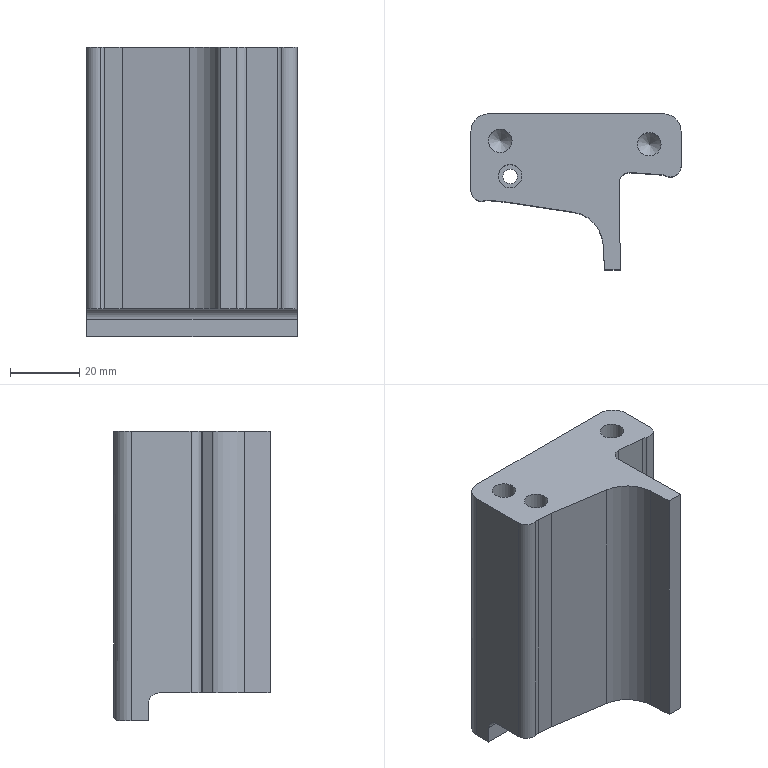Part | NX | features solid 2 | 1 solid | 32 faces | box 60.587 x 45.023 x 83.5 mm | volume 117737 mm3 | cylinder 15 | plane 14 | cone 3 | commonest cylinder face diameters 6 x6 6.8 x3 10 x2 2 x1 4.2 x1 5.2 x1
STEP:
#1=CARTESIAN_POINT('',(40.263,90.,-5.5));
#2=VERTEX_POINT('',#1);
#3=CARTESIAN_POINT('',(42.363,90.,-5.5));
#4=DIRECTION('',(0.,0.,-1.));
#5=DIRECTION('',(-1.,0.,0.));
#6=AXIS2_PLACEMENT_3D('',#3,#4,#5);
#7=CIRCLE('',#6,2.1);
#8=EDGE_CURVE('',#2,#2,#7,.T.);
#9=ORIENTED_EDGE('',*,*,#8,.F.);
#10=EDGE_LOOP('',(#9));
#11=FACE_BOUND('',#10,.T.);
#12=CARTESIAN_POINT('',(74.154,62.977,-5.5));
#13=VERTEX_POINT('',#12);
#14=CARTESIAN_POINT('',(69.599,62.977,-5.5));
#15=VERTEX_POINT('',#14);
#16=CARTESIAN_POINT('',(34.069,62.977,-5.5));
#17=DIRECTION('',(1.,0.,0.));
#18=VECTOR('',#17,1000.);
#19=LINE('',#16,#18);
#20=EDGE_CURVE('',#13,#15,#19,.F.);
#21=ORIENTED_EDGE('',*,*,#20,.T.);
#22=CARTESIAN_POINT('',(69.171,70.288,-5.5));
#23=VERTEX_POINT('',#22);
#24=CARTESIAN_POINT('',(69.651,62.096,-5.5));
#25=DIRECTION('',(-0.05848,0.9983,0.));
#26=VECTOR('',#25,1000.);
#27=LINE('',#24,#26);
#28=EDGE_CURVE('',#15,#23,#27,.T.);
#29=ORIENTED_EDGE('',*,*,#28,.T.);
#30=CARTESIAN_POINT('',(60.68,79.591,-5.5));
#31=VERTEX_POINT('',#30);
#32=CARTESIAN_POINT('',(59.188,69.703,-5.5));
#33=DIRECTION('',(0.,0.,1.));
#34=DIRECTION('',(1.,0.,0.));
#35=AXIS2_PLACEMENT_3D('',#32,#33,#34);
#36=CIRCLE('',#35,10.);
#37=EDGE_CURVE('',#23,#31,#36,.T.);
#38=ORIENTED_EDGE('',*,*,#37,.T.);
#39=CARTESIAN_POINT('',(41.179,82.535,-5.5));
#40=VERTEX_POINT('',#39);
#41=CARTESIAN_POINT('',(60.68,79.591,-5.5));
#42=DIRECTION('',(-0.9888,0.1493,0.));
#43=VECTOR('',#42,1000.);
#44=LINE('',#41,#43);
#45=EDGE_CURVE('',#31,#40,#44,.T.);
#46=ORIENTED_EDGE('',*,*,#45,.T.);
#47=CARTESIAN_POINT('',(36.197,83.04,-5.5));
#48=VERTEX_POINT('',#47);
#49=CARTESIAN_POINT('',(41.179,82.535,-5.5));
#50=DIRECTION('',(-0.9949,0.1009,0.));
#51=VECTOR('',#50,1000.);
#52=LINE('',#49,#51);
#53=EDGE_CURVE('',#40,#48,#52,.T.);
#54=ORIENTED_EDGE('',*,*,#53,.T.);
#55=CARTESIAN_POINT('',(34.982,82.913,-5.5));
#56=VERTEX_POINT('',#55);
#57=CARTESIAN_POINT('',(35.894,80.055,-5.5));
#58=DIRECTION('',(0.,0.,1.));
#59=DIRECTION('',(1.,0.,0.));
#60=AXIS2_PLACEMENT_3D('',#57,#58,#59);
#61=CIRCLE('',#60,3.);
#62=EDGE_CURVE('',#48,#56,#61,.T.);
#63=ORIENTED_EDGE('',*,*,#62,.T.);
#64=CARTESIAN_POINT('',(31.069,85.771,-5.5));
#65=VERTEX_POINT('',#64);
#66=CARTESIAN_POINT('',(34.069,85.771,-5.5));
#67=DIRECTION('',(0.,0.,-1.));
#68=DIRECTION('',(1.,0.,0.));
#69=AXIS2_PLACEMENT_3D('',#66,#67,#68);
#70=CIRCLE('',#69,3.);
#71=EDGE_CURVE('',#56,#65,#70,.T.);
#72=ORIENTED_EDGE('',*,*,#71,.T.);
#73=CARTESIAN_POINT('',(31.069,95.,-5.5));
#74=VERTEX_POINT('',#73);
#75=CARTESIAN_POINT('',(31.069,85.771,-5.5));
#76=DIRECTION('',(0.,1.,0.));
#77=VECTOR('',#76,1000.);
#78=LINE('',#75,#77);
#79=EDGE_CURVE('',#65,#74,#78,.T.);
#80=ORIENTED_EDGE('',*,*,#79,.T.);
#81=CARTESIAN_POINT('',(91.657,95.,-5.5));
#82=VERTEX_POINT('',#81);
#83=CARTESIAN_POINT('',(34.069,95.,-5.5));
#84=DIRECTION('',(1.,0.,0.));
#85=VECTOR('',#84,1000.);
#86=LINE('',#83,#85);
#87=EDGE_CURVE('',#74,#82,#86,.T.);
#88=ORIENTED_EDGE('',*,*,#87,.T.);
#89=CARTESIAN_POINT('',(91.657,92.731,-5.5));
#90=VERTEX_POINT('',#89);
#91=CARTESIAN_POINT('',(91.657,109.703,-5.5));
#92=DIRECTION('',(0.,-1.,0.));
#93=VECTOR('',#92,1000.);
#94=LINE('',#91,#93);
#95=EDGE_CURVE('',#82,#90,#94,.T.);
#96=ORIENTED_EDGE('',*,*,#95,.T.);
#97=CARTESIAN_POINT('',(87.27,90.071,-5.5));
#98=VERTEX_POINT('',#97);
#99=CARTESIAN_POINT('',(88.657,92.731,-5.5));
#100=DIRECTION('',(0.,0.,-1.));
#101=DIRECTION('',(1.,0.,0.));
#102=AXIS2_PLACEMENT_3D('',#99,#100,#101);
#103=CIRCLE('',#102,3.);
#104=EDGE_CURVE('',#90,#98,#103,.T.);
#105=ORIENTED_EDGE('',*,*,#104,.T.);
#106=CARTESIAN_POINT('',(86.093,90.403,-5.5));
#107=VERTEX_POINT('',#106);
#108=CARTESIAN_POINT('',(85.883,87.411,-5.5));
#109=DIRECTION('',(0.,0.,1.));
#110=DIRECTION('',(1.,0.,0.));
#111=AXIS2_PLACEMENT_3D('',#108,#109,#110);
#112=CIRCLE('',#111,3.);
#113=EDGE_CURVE('',#98,#107,#112,.T.);
#114=ORIENTED_EDGE('',*,*,#113,.T.);
#115=CARTESIAN_POINT('',(77.047,91.037,-5.5));
#116=VERTEX_POINT('',#115);
#117=CARTESIAN_POINT('',(86.093,90.403,-5.5));
#118=DIRECTION('',(-0.9976,0.06991,0.));
#119=VECTOR('',#118,1000.);
#120=LINE('',#117,#119);
#121=EDGE_CURVE('',#107,#116,#120,.T.);
#122=ORIENTED_EDGE('',*,*,#121,.T.);
#123=CARTESIAN_POINT('',(73.838,88.007,-5.5));
#124=VERTEX_POINT('',#123);
#125=CARTESIAN_POINT('',(76.838,88.044,-5.5));
#126=DIRECTION('',(0.,0.,1.));
#127=DIRECTION('',(1.,0.,0.));
#128=AXIS2_PLACEMENT_3D('',#125,#126,#127);
#129=CIRCLE('',#128,3.);
#130=EDGE_CURVE('',#116,#124,#129,.T.);
#131=ORIENTED_EDGE('',*,*,#130,.T.);
#132=CARTESIAN_POINT('',(73.838,88.007,-5.5));
#133=DIRECTION('',(0.01263,-0.9999,0.));
#134=VECTOR('',#133,1000.);
#135=LINE('',#132,#134);
#136=EDGE_CURVE('',#124,#13,#135,.T.);
#137=ORIENTED_EDGE('',*,*,#136,.T.);
#138=EDGE_LOOP('',(#21,#29,#38,#46,#54,#63,#72,#80,#88,#96,#105,#114,#122,#131,#137));
#139=FACE_BOUND('',#138,.T.);
#140=CARTESIAN_POINT('',(58.763,91.,-5.5));
#141=VERTEX_POINT('',#140);
#142=CARTESIAN_POINT('',(61.363,91.,-5.5));
#143=DIRECTION('',(0.,0.,-1.));
#144=DIRECTION('',(-1.,0.,0.));
#145=AXIS2_PLACEMENT_3D('',#142,#143,#144);
#146=CIRCLE('',#145,2.6);
#147=EDGE_CURVE('',#141,#141,#146,.F.);
#148=ORIENTED_EDGE('',*,*,#147,.T.);
#149=EDGE_LOOP('',(#148));
#150=FACE_BOUND('',#149,.T.);
#151=CARTESIAN_POINT('',(34.069,110.84,-5.5));
#152=DIRECTION('',(0.,0.,-1.));
#153=DIRECTION('',(-1.,0.,0.));
#154=AXIS2_PLACEMENT_3D('',#151,#152,#153);
#155=PLANE('',#154);
#156=ADVANCED_FACE('',(#11,#139,#150),#155,.T.);
#157=CARTESIAN_POINT('',(91.657,98.,-13.5));
#158=VERTEX_POINT('',#157);
#159=CARTESIAN_POINT('',(91.657,103.,-13.5));
#160=VERTEX_POINT('',#159);
#161=CARTESIAN_POINT('',(91.657,98.,-13.5));
#162=DIRECTION('',(0.,1.,0.));
#163=VECTOR('',#162,1000.);
#164=LINE('',#161,#163);
#165=EDGE_CURVE('',#158,#160,#164,.T.);
#166=ORIENTED_EDGE('',*,*,#165,.F.);
#167=CARTESIAN_POINT('',(31.069,98.,-13.5));
#168=VERTEX_POINT('',#167);
#169=CARTESIAN_POINT('',(34.069,98.,-13.5));
#170=DIRECTION('',(1.,0.,0.));
#171=VECTOR('',#170,1000.);
#172=LINE('',#169,#171);
#173=EDGE_CURVE('',#168,#158,#172,.T.);
#174=ORIENTED_EDGE('',*,*,#173,.F.);
#175=CARTESIAN_POINT('',(31.069,103.,-13.5));
#176=VERTEX_POINT('',#175);
#177=CARTESIAN_POINT('',(31.069,98.,-13.5));
#178=DIRECTION('',(0.,1.,0.));
#179=VECTOR('',#178,1000.);
#180=LINE('',#177,#179);
#181=EDGE_CURVE('',#168,#176,#180,.T.);
#182=ORIENTED_EDGE('',*,*,#181,.T.);
#183=CARTESIAN_POINT('',(33.069,107.,-13.5));
#184=VERTEX_POINT('',#183);
#185=CARTESIAN_POINT('',(36.069,103.,-13.5));
#186=DIRECTION('',(0.,0.,1.));
#187=DIRECTION('',(1.,0.,0.));
#188=AXIS2_PLACEMENT_3D('',#185,#186,#187);
#189=CIRCLE('',#188,5.);
#190=EDGE_CURVE('',#176,#184,#189,.F.);
#191=ORIENTED_EDGE('',*,*,#190,.T.);
#192=CARTESIAN_POINT('',(89.657,107.,-13.5));
#193=VERTEX_POINT('',#192);
#194=CARTESIAN_POINT('',(86.657,107.,-13.5));
#195=DIRECTION('',(-1.,0.,0.));
#196=VECTOR('',#195,1000.);
#197=LINE('',#194,#196);
#198=EDGE_CURVE('',#184,#193,#197,.F.);
#199=ORIENTED_EDGE('',*,*,#198,.T.);
#200=CARTESIAN_POINT('',(86.657,103.,-13.5));
#201=DIRECTION('',(0.,0.,1.));
#202=DIRECTION('',(1.,0.,0.));
#203=AXIS2_PLACEMENT_3D('',#200,#201,#202);
#204=CIRCLE('',#203,5.);
#205=EDGE_CURVE('',#193,#160,#204,.F.);
#206=ORIENTED_EDGE('',*,*,#205,.T.);
#207=EDGE_LOOP('',(#166,#174,#182,#191,#199,#206));
#208=FACE_BOUND('',#207,.T.);
#209=CARTESIAN_POINT('',(34.069,98.,-13.5));
#210=DIRECTION('',(0.,0.,1.));
#211=DIRECTION('',(1.,0.,0.));
#212=AXIS2_PLACEMENT_3D('',#209,#210,#211);
#213=PLANE('',#212);
#214=ADVANCED_FACE('',(#208),#213,.F.);
#215=CARTESIAN_POINT('',(42.9,100.2,70.));
#216=VERTEX_POINT('',#215);
#217=CARTESIAN_POINT('',(39.5,100.2,70.));
#218=DIRECTION('',(0.,0.,-1.));
#219=DIRECTION('',(1.,0.,0.));
#220=AXIS2_PLACEMENT_3D('',#217,#218,#219);
#221=CIRCLE('',#220,3.4);
#222=EDGE_CURVE('',#216,#216,#221,.T.);
#223=ORIENTED_EDGE('',*,*,#222,.T.);
#224=EDGE_LOOP('',(#223));
#225=FACE_BOUND('',#224,.T.);
#226=CARTESIAN_POINT('',(74.154,62.977,70.));
#227=VERTEX_POINT('',#226);
#228=CARTESIAN_POINT('',(69.599,62.977,70.));
#229=VERTEX_POINT('',#228);
#230=CARTESIAN_POINT('',(-37.5,62.977,70.));
#231=DIRECTION('',(-1.,0.,0.));
#232=VECTOR('',#231,1000.);
#233=LINE('',#230,#232);
#234=EDGE_CURVE('',#227,#229,#233,.T.);
#235=ORIENTED_EDGE('',*,*,#234,.F.);
#236=CARTESIAN_POINT('',(73.838,88.007,70.));
#237=VERTEX_POINT('',#236);
#238=CARTESIAN_POINT('',(73.838,88.007,70.));
#239=DIRECTION('',(0.01263,-0.9999,0.));
#240=VECTOR('',#239,1000.);
#241=LINE('',#238,#240);
#242=EDGE_CURVE('',#237,#227,#241,.T.);
#243=ORIENTED_EDGE('',*,*,#242,.F.);
#244=CARTESIAN_POINT('',(77.047,91.037,70.));
#245=VERTEX_POINT('',#244);
#246=CARTESIAN_POINT('',(76.838,88.044,70.));
#247=DIRECTION('',(0.,0.,1.));
#248=DIRECTION('',(1.,0.,0.));
#249=AXIS2_PLACEMENT_3D('',#246,#247,#248);
#250=CIRCLE('',#249,3.);
#251=EDGE_CURVE('',#245,#237,#250,.T.);
#252=ORIENTED_EDGE('',*,*,#251,.F.);
#253=CARTESIAN_POINT('',(86.093,90.403,70.));
#254=VERTEX_POINT('',#253);
#255=CARTESIAN_POINT('',(86.093,90.403,70.));
#256=DIRECTION('',(-0.9976,0.06991,0.));
#257=VECTOR('',#256,1000.);
#258=LINE('',#255,#257);
#259=EDGE_CURVE('',#254,#245,#258,.T.);
#260=ORIENTED_EDGE('',*,*,#259,.F.);
#261=CARTESIAN_POINT('',(87.27,90.071,70.));
#262=VERTEX_POINT('',#261);
#263=CARTESIAN_POINT('',(85.883,87.411,70.));
#264=DIRECTION('',(0.,0.,1.));
#265=DIRECTION('',(1.,0.,0.));
#266=AXIS2_PLACEMENT_3D('',#263,#264,#265);
#267=CIRCLE('',#266,3.);
#268=EDGE_CURVE('',#262,#254,#267,.T.);
#269=ORIENTED_EDGE('',*,*,#268,.F.);
#270=CARTESIAN_POINT('',(91.657,92.731,70.));
#271=VERTEX_POINT('',#270);
#272=CARTESIAN_POINT('',(88.657,92.731,70.));
#273=DIRECTION('',(0.,0.,1.));
#274=DIRECTION('',(1.,0.,0.));
#275=AXIS2_PLACEMENT_3D('',#272,#273,#274);
#276=CIRCLE('',#275,3.);
#277=EDGE_CURVE('',#271,#262,#276,.F.);
#278=ORIENTED_EDGE('',*,*,#277,.F.);
#279=CARTESIAN_POINT('',(91.657,103.,70.));
#280=VERTEX_POINT('',#279);
#281=CARTESIAN_POINT('',(91.657,109.703,70.));
#282=DIRECTION('',(0.,-1.,0.));
#283=VECTOR('',#282,1000.);
#284=LINE('',#281,#283);
#285=EDGE_CURVE('',#280,#271,#284,.T.);
#286=ORIENTED_EDGE('',*,*,#285,.F.);
#287=CARTESIAN_POINT('',(86.657,108.,70.));
#288=VERTEX_POINT('',#287);
#289=CARTESIAN_POINT('',(86.657,103.,70.));
#290=DIRECTION('',(0.,0.,1.));
#291=DIRECTION('',(1.,0.,0.));
#292=AXIS2_PLACEMENT_3D('',#289,#290,#291);
#293=CIRCLE('',#292,5.);
#294=EDGE_CURVE('',#288,#280,#293,.F.);
#295=ORIENTED_EDGE('',*,*,#294,.F.);
#296=CARTESIAN_POINT('',(36.069,108.,70.));
#297=VERTEX_POINT('',#296);
#298=CARTESIAN_POINT('',(34.069,108.,70.));
#299=DIRECTION('',(1.,0.,0.));
#300=VECTOR('',#299,1000.);
#301=LINE('',#298,#300);
#302=EDGE_CURVE('',#297,#288,#301,.T.);
#303=ORIENTED_EDGE('',*,*,#302,.F.);
#304=CARTESIAN_POINT('',(31.069,103.,70.));
#305=VERTEX_POINT('',#304);
#306=CARTESIAN_POINT('',(36.069,103.,70.));
#307=DIRECTION('',(0.,0.,1.));
#308=DIRECTION('',(1.,0.,0.));
#309=AXIS2_PLACEMENT_3D('',#306,#307,#308);
#310=CIRCLE('',#309,5.);
#311=EDGE_CURVE('',#305,#297,#310,.F.);
#312=ORIENTED_EDGE('',*,*,#311,.F.);
#313=CARTESIAN_POINT('',(31.069,85.771,70.));
#314=VERTEX_POINT('',#313);
#315=CARTESIAN_POINT('',(31.069,85.771,70.));
#316=DIRECTION('',(0.,1.,0.));
#317=VECTOR('',#316,1000.);
#318=LINE('',#315,#317);
#319=EDGE_CURVE('',#314,#305,#318,.T.);
#320=ORIENTED_EDGE('',*,*,#319,.F.);
#321=CARTESIAN_POINT('',(34.982,82.913,70.));
#322=VERTEX_POINT('',#321);
#323=CARTESIAN_POINT('',(34.069,85.771,70.));
#324=DIRECTION('',(0.,0.,1.));
#325=DIRECTION('',(1.,0.,0.));
#326=AXIS2_PLACEMENT_3D('',#323,#324,#325);
#327=CIRCLE('',#326,3.);
#328=EDGE_CURVE('',#322,#314,#327,.F.);
#329=ORIENTED_EDGE('',*,*,#328,.F.);
#330=CARTESIAN_POINT('',(36.197,83.04,70.));
#331=VERTEX_POINT('',#330);
#332=CARTESIAN_POINT('',(35.894,80.055,70.));
#333=DIRECTION('',(0.,0.,1.));
#334=DIRECTION('',(1.,0.,0.));
#335=AXIS2_PLACEMENT_3D('',#332,#333,#334);
#336=CIRCLE('',#335,3.);
#337=EDGE_CURVE('',#331,#322,#336,.T.);
#338=ORIENTED_EDGE('',*,*,#337,.F.);
#339=CARTESIAN_POINT('',(41.179,82.535,70.));
#340=VERTEX_POINT('',#339);
#341=CARTESIAN_POINT('',(41.179,82.535,70.));
#342=DIRECTION('',(-0.9949,0.1009,0.));
#343=VECTOR('',#342,1000.);
#344=LINE('',#341,#343);
#345=EDGE_CURVE('',#340,#331,#344,.T.);
#346=ORIENTED_EDGE('',*,*,#345,.F.);
#347=CARTESIAN_POINT('',(60.68,79.591,70.));
#348=VERTEX_POINT('',#347);
#349=CARTESIAN_POINT('',(60.68,79.591,70.));
#350=DIRECTION('',(-0.9888,0.1493,0.));
#351=VECTOR('',#350,1000.);
#352=LINE('',#349,#351);
#353=EDGE_CURVE('',#348,#340,#352,.T.);
#354=ORIENTED_EDGE('',*,*,#353,.F.);
#355=CARTESIAN_POINT('',(69.171,70.288,70.));
#356=VERTEX_POINT('',#355);
#357=CARTESIAN_POINT('',(59.188,69.703,70.));
#358=DIRECTION('',(0.,0.,1.));
#359=DIRECTION('',(1.,0.,0.));
#360=AXIS2_PLACEMENT_3D('',#357,#358,#359);
#361=CIRCLE('',#360,10.);
#362=EDGE_CURVE('',#348,#356,#361,.F.);
#363=ORIENTED_EDGE('',*,*,#362,.T.);
#364=CARTESIAN_POINT('',(69.651,62.096,70.));
#365=DIRECTION('',(-0.05848,0.9983,0.));
#366=VECTOR('',#365,1000.);
#367=LINE('',#364,#366);
#368=EDGE_CURVE('',#356,#229,#367,.F.);
#369=ORIENTED_EDGE('',*,*,#368,.T.);
#370=EDGE_LOOP('',(#235,#243,#252,#260,#269,#278,#286,#295,#303,#312,#320,#329,#338,#346,#354,#363,#369));
#371=FACE_BOUND('',#370,.T.);
#372=CARTESIAN_POINT('',(45.763,90.,70.));
#373=VERTEX_POINT('',#372);
#374=CARTESIAN_POINT('',(42.363,90.,70.));
#375=DIRECTION('',(0.,0.,1.));
#376=DIRECTION('',(1.,0.,0.));
#377=AXIS2_PLACEMENT_3D('',#374,#375,#376);
#378=CIRCLE('',#377,3.4);
#379=EDGE_CURVE('',#373,#373,#378,.T.);
#380=ORIENTED_EDGE('',*,*,#379,.F.);
#381=EDGE_LOOP('',(#380));
#382=FACE_BOUND('',#381,.T.);
#383=CARTESIAN_POINT('',(85.9,99.2,70.));
#384=VERTEX_POINT('',#383);
#385=CARTESIAN_POINT('',(82.5,99.2,70.));
#386=DIRECTION('',(0.,0.,-1.));
#387=DIRECTION('',(1.,0.,0.));
#388=AXIS2_PLACEMENT_3D('',#385,#386,#387);
#389=CIRCLE('',#388,3.4);
#390=EDGE_CURVE('',#384,#384,#389,.T.);
#391=ORIENTED_EDGE('',*,*,#390,.T.);
#392=EDGE_LOOP('',(#391));
#393=FACE_BOUND('',#392,.T.);
#394=CARTESIAN_POINT('',(-37.5,0.,70.));
#395=DIRECTION('',(0.,0.,1.));
#396=DIRECTION('',(1.,0.,0.));
#397=AXIS2_PLACEMENT_3D('',#394,#395,#396);
#398=PLANE('',#397);
#399=ADVANCED_FACE('',(#225,#371,#382,#393),#398,.T.);
#400=ORIENTED_EDGE('',*,*,#173,.T.);
#401=CARTESIAN_POINT('',(91.657,98.,-8.5));
#402=VERTEX_POINT('',#401);
#403=CARTESIAN_POINT('',(91.657,98.,40.));
#404=DIRECTION('',(0.,0.,-1.));
#405=VECTOR('',#404,1000.);
#406=LINE('',#403,#405);
#407=EDGE_CURVE('',#402,#158,#406,.T.);
#408=ORIENTED_EDGE('',*,*,#407,.F.);
#409=CARTESIAN_POINT('',(31.069,98.,-8.5));
#410=VERTEX_POINT('',#409);
#411=CARTESIAN_POINT('',(34.069,98.,-8.5));
#412=DIRECTION('',(1.,0.,0.));
#413=VECTOR('',#412,1000.);
#414=LINE('',#411,#413);
#415=EDGE_CURVE('',#402,#410,#414,.F.);
#416=ORIENTED_EDGE('',*,*,#415,.T.);
#417=CARTESIAN_POINT('',(31.069,98.,40.));
#418=DIRECTION('',(0.,0.,-1.));
#419=VECTOR('',#418,1000.);
#420=LINE('',#417,#419);
#421=EDGE_CURVE('',#410,#168,#420,.T.);
#422=ORIENTED_EDGE('',*,*,#421,.T.);
#423=EDGE_LOOP('',(#400,#408,#416,#422));
#424=FACE_BOUND('',#423,.T.);
#425=CARTESIAN_POINT('',(34.069,98.,40.));
#426=DIRECTION('',(0.,1.,0.));
#427=DIRECTION('',(0.,0.,1.));
#428=AXIS2_PLACEMENT_3D('',#425,#426,#427);
#429=PLANE('',#428);
#430=ADVANCED_FACE('',(#424),#429,.F.);
#431=CARTESIAN_POINT('',(91.657,95.,-8.5));
#432=DIRECTION('',(1.,0.,0.));
#433=DIRECTION('',(0.,1.,0.));
#434=AXIS2_PLACEMENT_3D('',#431,#432,#433);
#435=CIRCLE('',#434,3.);
#436=EDGE_CURVE('',#82,#402,#435,.F.);
#437=ORIENTED_EDGE('',*,*,#436,.F.);
#438=ORIENTED_EDGE('',*,*,#87,.F.);
#439=CARTESIAN_POINT('',(31.069,95.,-8.5));
#440=DIRECTION('',(-1.,0.,0.));
#441=DIRECTION('',(0.,-1.,0.));
#442=AXIS2_PLACEMENT_3D('',#439,#440,#441);
#443=CIRCLE('',#442,3.);
#444=EDGE_CURVE('',#410,#74,#443,.F.);
#445=ORIENTED_EDGE('',*,*,#444,.F.);
#446=ORIENTED_EDGE('',*,*,#415,.F.);
#447=EDGE_LOOP('',(#437,#438,#445,#446));
#448=FACE_BOUND('',#447,.T.);
#449=CARTESIAN_POINT('',(34.069,95.,-8.5));
#450=DIRECTION('',(1.,0.,0.));
#451=DIRECTION('',(0.,0.,-1.));
#452=AXIS2_PLACEMENT_3D('',#449,#450,#451);
#453=CYLINDRICAL_SURFACE('',#452,3.);
#454=ADVANCED_FACE('',(#448),#453,.F.);
#455=CARTESIAN_POINT('',(31.069,85.771,40.));
#456=DIRECTION('',(0.,0.,-1.));
#457=VECTOR('',#456,1000.);
#458=LINE('',#455,#457);
#459=EDGE_CURVE('',#314,#65,#458,.T.);
#460=ORIENTED_EDGE('',*,*,#459,.F.);
#461=ORIENTED_EDGE('',*,*,#319,.T.);
#462=CARTESIAN_POINT('',(31.069,103.,40.));
#463=DIRECTION('',(0.,0.,-1.));
#464=VECTOR('',#463,1000.);
#465=LINE('',#462,#464);
#466=EDGE_CURVE('',#305,#176,#465,.T.);
#467=ORIENTED_EDGE('',*,*,#466,.T.);
#468=ORIENTED_EDGE('',*,*,#181,.F.);
#469=ORIENTED_EDGE('',*,*,#421,.F.);
#470=ORIENTED_EDGE('',*,*,#444,.T.);
#471=ORIENTED_EDGE('',*,*,#79,.F.);
#472=EDGE_LOOP('',(#460,#461,#467,#468,#469,#470,#471));
#473=FACE_BOUND('',#472,.T.);
#474=CARTESIAN_POINT('',(31.069,85.771,40.));
#475=DIRECTION('',(-1.,0.,0.));
#476=DIRECTION('',(0.,-1.,0.));
#477=AXIS2_PLACEMENT_3D('',#474,#475,#476);
#478=PLANE('',#477);
#479=ADVANCED_FACE('',(#473),#478,.T.);
#480=CARTESIAN_POINT('',(34.982,82.913,40.));
#481=DIRECTION('',(0.,0.,-1.));
#482=VECTOR('',#481,1000.);
#483=LINE('',#480,#482);
#484=EDGE_CURVE('',#322,#56,#483,.T.);
#485=ORIENTED_EDGE('',*,*,#484,.F.);
#486=ORIENTED_EDGE('',*,*,#328,.T.);
#487=ORIENTED_EDGE('',*,*,#459,.T.);
#488=ORIENTED_EDGE('',*,*,#71,.F.);
#489=EDGE_LOOP('',(#485,#486,#487,#488));
#490=FACE_BOUND('',#489,.T.);
#491=CARTESIAN_POINT('',(34.069,85.771,40.));
#492=DIRECTION('',(0.,0.,-1.));
#493=DIRECTION('',(-1.,0.,0.));
#494=AXIS2_PLACEMENT_3D('',#491,#492,#493);
#495=CYLINDRICAL_SURFACE('',#494,3.);
#496=ADVANCED_FACE('',(#490),#495,.T.);
#497=CARTESIAN_POINT('',(36.197,83.04,40.));
#498=DIRECTION('',(0.,0.,-1.));
#499=VECTOR('',#498,1000.);
#500=LINE('',#497,#499);
#501=EDGE_CURVE('',#331,#48,#500,.T.);
#502=ORIENTED_EDGE('',*,*,#501,.F.);
#503=ORIENTED_EDGE('',*,*,#337,.T.);
#504=ORIENTED_EDGE('',*,*,#484,.T.);
#505=ORIENTED_EDGE('',*,*,#62,.F.);
#506=EDGE_LOOP('',(#502,#503,#504,#505));
#507=FACE_BOUND('',#506,.T.);
#508=CARTESIAN_POINT('',(35.894,80.055,40.));
#509=DIRECTION('',(0.,0.,-1.));
#510=DIRECTION('',(-1.,0.,0.));
#511=AXIS2_PLACEMENT_3D('',#508,#509,#510);
#512=CYLINDRICAL_SURFACE('',#511,3.);
#513=ADVANCED_FACE('',(#507),#512,.F.);
#514=CARTESIAN_POINT('',(41.179,82.535,40.));
#515=DIRECTION('',(0.,0.,-1.));
#516=VECTOR('',#515,1000.);
#517=LINE('',#514,#516);
#518=EDGE_CURVE('',#340,#40,#517,.T.);
#519=ORIENTED_EDGE('',*,*,#518,.F.);
#520=ORIENTED_EDGE('',*,*,#345,.T.);
#521=ORIENTED_EDGE('',*,*,#501,.T.);
#522=ORIENTED_EDGE('',*,*,#53,.F.);
#523=EDGE_LOOP('',(#519,#520,#521,#522));
#524=FACE_BOUND('',#523,.T.);
#525=CARTESIAN_POINT('',(41.179,82.535,40.));
#526=DIRECTION('',(-0.1009,-0.9949,0.));
#527=DIRECTION('',(0.9949,-0.1009,0.));
#528=AXIS2_PLACEMENT_3D('',#525,#526,#527);
#529=PLANE('',#528);
#530=ADVANCED_FACE('',(#524),#529,.T.);
#531=ORIENTED_EDGE('',*,*,#353,.T.);
#532=ORIENTED_EDGE('',*,*,#518,.T.);
#533=ORIENTED_EDGE('',*,*,#45,.F.);
#534=CARTESIAN_POINT('',(60.68,79.591,40.));
#535=DIRECTION('',(0.,0.,-1.));
#536=VECTOR('',#535,1000.);
#537=LINE('',#534,#536);
#538=EDGE_CURVE('',#348,#31,#537,.T.);
#539=ORIENTED_EDGE('',*,*,#538,.F.);
#540=EDGE_LOOP('',(#531,#532,#533,#539));
#541=FACE_BOUND('',#540,.T.);
#542=CARTESIAN_POINT('',(60.68,79.591,40.));
#543=DIRECTION('',(-0.1493,-0.9888,0.));
#544=DIRECTION('',(0.9888,-0.1493,0.));
#545=AXIS2_PLACEMENT_3D('',#542,#543,#544);
#546=PLANE('',#545);
#547=ADVANCED_FACE('',(#541),#546,.T.);
#548=ORIENTED_EDGE('',*,*,#362,.F.);
#549=ORIENTED_EDGE('',*,*,#538,.T.);
#550=ORIENTED_EDGE('',*,*,#37,.F.);
#551=CARTESIAN_POINT('',(69.171,70.288,40.));
#552=DIRECTION('',(0.,0.,-1.));
#553=VECTOR('',#552,1000.);
#554=LINE('',#551,#553);
#555=EDGE_CURVE('',#356,#23,#554,.T.);
#556=ORIENTED_EDGE('',*,*,#555,.F.);
#557=EDGE_LOOP('',(#548,#549,#550,#556));
#558=FACE_BOUND('',#557,.T.);
#559=CARTESIAN_POINT('',(59.188,69.703,40.));
#560=DIRECTION('',(0.,0.,-1.));
#561=DIRECTION('',(-1.,0.,0.));
#562=AXIS2_PLACEMENT_3D('',#559,#560,#561);
#563=CYLINDRICAL_SURFACE('',#562,10.);
#564=ADVANCED_FACE('',(#558),#563,.F.);
#565=CARTESIAN_POINT('',(69.599,62.977,40.));
#566=DIRECTION('',(0.,0.,-1.));
#567=VECTOR('',#566,1000.);
#568=LINE('',#565,#567);
#569=EDGE_CURVE('',#15,#229,#568,.F.);
#570=ORIENTED_EDGE('',*,*,#569,.T.);
#571=ORIENTED_EDGE('',*,*,#368,.F.);
#572=ORIENTED_EDGE('',*,*,#555,.T.);
#573=ORIENTED_EDGE('',*,*,#28,.F.);
#574=EDGE_LOOP('',(#570,#571,#572,#573));
#575=FACE_BOUND('',#574,.T.);
#576=CARTESIAN_POINT('',(69.651,62.096,40.));
#577=DIRECTION('',(-0.9983,-0.05848,0.));
#578=DIRECTION('',(0.05848,-0.9983,0.));
#579=AXIS2_PLACEMENT_3D('',#576,#577,#578);
#580=PLANE('',#579);
#581=ADVANCED_FACE('',(#575),#580,.T.);
#582=CARTESIAN_POINT('',(74.154,62.977,40.));
#583=DIRECTION('',(0.,0.,1.));
#584=VECTOR('',#583,1000.);
#585=LINE('',#582,#584);
#586=EDGE_CURVE('',#13,#227,#585,.T.);
#587=ORIENTED_EDGE('',*,*,#586,.F.);
#588=ORIENTED_EDGE('',*,*,#136,.F.);
#589=CARTESIAN_POINT('',(73.838,88.007,40.));
#590=DIRECTION('',(0.,0.,-1.));
#591=VECTOR('',#590,1000.);
#592=LINE('',#589,#591);
#593=EDGE_CURVE('',#237,#124,#592,.T.);
#594=ORIENTED_EDGE('',*,*,#593,.F.);
#595=ORIENTED_EDGE('',*,*,#242,.T.);
#596=EDGE_LOOP('',(#587,#588,#594,#595));
#597=FACE_BOUND('',#596,.T.);
#598=CARTESIAN_POINT('',(73.838,88.007,40.));
#599=DIRECTION('',(0.9999,0.01263,0.));
#600=DIRECTION('',(-0.01263,0.9999,0.));
#601=AXIS2_PLACEMENT_3D('',#598,#599,#600);
#602=PLANE('',#601);
#603=ADVANCED_FACE('',(#597),#602,.T.);
#604=CARTESIAN_POINT('',(77.047,91.037,40.));
#605=DIRECTION('',(0.,0.,-1.));
#606=VECTOR('',#605,1000.);
#607=LINE('',#604,#606);
#608=EDGE_CURVE('',#245,#116,#607,.T.);
#609=ORIENTED_EDGE('',*,*,#608,.F.);
#610=ORIENTED_EDGE('',*,*,#251,.T.);
#611=ORIENTED_EDGE('',*,*,#593,.T.);
#612=ORIENTED_EDGE('',*,*,#130,.F.);
#613=EDGE_LOOP('',(#609,#610,#611,#612));
#614=FACE_BOUND('',#613,.T.);
#615=CARTESIAN_POINT('',(76.838,88.044,40.));
#616=DIRECTION('',(0.,0.,-1.));
#617=DIRECTION('',(-1.,0.,0.));
#618=AXIS2_PLACEMENT_3D('',#615,#616,#617);
#619=CYLINDRICAL_SURFACE('',#618,3.);
#620=ADVANCED_FACE('',(#614),#619,.F.);
#621=CARTESIAN_POINT('',(86.093,90.403,40.));
#622=DIRECTION('',(0.,0.,-1.));
#623=VECTOR('',#622,1000.);
#624=LINE('',#621,#623);
#625=EDGE_CURVE('',#254,#107,#624,.T.);
#626=ORIENTED_EDGE('',*,*,#625,.F.);
#627=ORIENTED_EDGE('',*,*,#259,.T.);
#628=ORIENTED_EDGE('',*,*,#608,.T.);
#629=ORIENTED_EDGE('',*,*,#121,.F.);
#630=EDGE_LOOP('',(#626,#627,#628,#629));
#631=FACE_BOUND('',#630,.T.);
#632=CARTESIAN_POINT('',(86.093,90.403,40.));
#633=DIRECTION('',(-0.06991,-0.9976,0.));
#634=DIRECTION('',(0.9976,-0.06991,0.));
#635=AXIS2_PLACEMENT_3D('',#632,#633,#634);
#636=PLANE('',#635);
#637=ADVANCED_FACE('',(#631),#636,.T.);
#638=CARTESIAN_POINT('',(87.27,90.071,40.));
#639=DIRECTION('',(0.,0.,-1.));
#640=VECTOR('',#639,1000.);
#641=LINE('',#638,#640);
#642=EDGE_CURVE('',#262,#98,#641,.T.);
#643=ORIENTED_EDGE('',*,*,#642,.F.);
#644=ORIENTED_EDGE('',*,*,#268,.T.);
#645=ORIENTED_EDGE('',*,*,#625,.T.);
#646=ORIENTED_EDGE('',*,*,#113,.F.);
#647=EDGE_LOOP('',(#643,#644,#645,#646));
#648=FACE_BOUND('',#647,.T.);
#649=CARTESIAN_POINT('',(85.883,87.411,40.));
#650=DIRECTION('',(0.,0.,-1.));
#651=DIRECTION('',(-1.,0.,0.));
#652=AXIS2_PLACEMENT_3D('',#649,#650,#651);
#653=CYLINDRICAL_SURFACE('',#652,3.);
#654=ADVANCED_FACE('',(#648),#653,.F.);
#655=CARTESIAN_POINT('',(91.657,92.731,40.));
#656=DIRECTION('',(0.,0.,-1.));
#657=VECTOR('',#656,1000.);
#658=LINE('',#655,#657);
#659=EDGE_CURVE('',#271,#90,#658,.T.);
#660=ORIENTED_EDGE('',*,*,#659,.F.);
#661=ORIENTED_EDGE('',*,*,#277,.T.);
#662=ORIENTED_EDGE('',*,*,#642,.T.);
#663=ORIENTED_EDGE('',*,*,#104,.F.);
#664=EDGE_LOOP('',(#660,#661,#662,#663));
#665=FACE_BOUND('',#664,.T.);
#666=CARTESIAN_POINT('',(88.657,92.731,40.));
#667=DIRECTION('',(0.,0.,-1.));
#668=DIRECTION('',(-1.,0.,0.));
#669=AXIS2_PLACEMENT_3D('',#666,#667,#668);
#670=CYLINDRICAL_SURFACE('',#669,3.);
#671=ADVANCED_FACE('',(#665),#670,.T.);
#672=CARTESIAN_POINT('',(91.657,103.,40.));
#673=DIRECTION('',(0.,0.,-1.));
#674=VECTOR('',#673,1000.);
#675=LINE('',#672,#674);
#676=EDGE_CURVE('',#160,#280,#675,.F.);
#677=ORIENTED_EDGE('',*,*,#676,.T.);
#678=ORIENTED_EDGE('',*,*,#285,.T.);
#679=ORIENTED_EDGE('',*,*,#659,.T.);
#680=ORIENTED_EDGE('',*,*,#95,.F.);
#681=ORIENTED_EDGE('',*,*,#436,.T.);
#682=ORIENTED_EDGE('',*,*,#407,.T.);
#683=ORIENTED_EDGE('',*,*,#165,.T.);
#684=EDGE_LOOP('',(#677,#678,#679,#680,#681,#682,#683));
#685=FACE_BOUND('',#684,.T.);
#686=CARTESIAN_POINT('',(91.657,109.703,40.));
#687=DIRECTION('',(1.,0.,0.));
#688=DIRECTION('',(0.,1.,0.));
#689=AXIS2_PLACEMENT_3D('',#686,#687,#688);
#690=PLANE('',#689);
#691=ADVANCED_FACE('',(#685),#690,.T.);
#692=CARTESIAN_POINT('',(36.069,108.,-12.5));
#693=VERTEX_POINT('',#692);
#694=CARTESIAN_POINT('',(36.069,108.,40.));
#695=DIRECTION('',(0.,0.,-1.));
#696=VECTOR('',#695,1000.);
#697=LINE('',#694,#696);
#698=EDGE_CURVE('',#693,#297,#697,.F.);
#699=ORIENTED_EDGE('',*,*,#698,.T.);
#700=ORIENTED_EDGE('',*,*,#302,.T.);
#701=CARTESIAN_POINT('',(86.657,108.,-12.5));
#702=VERTEX_POINT('',#701);
#703=CARTESIAN_POINT('',(86.657,108.,40.));
#704=DIRECTION('',(0.,0.,-1.));
#705=VECTOR('',#704,1000.);
#706=LINE('',#703,#705);
#707=EDGE_CURVE('',#288,#702,#706,.T.);
#708=ORIENTED_EDGE('',*,*,#707,.T.);
#709=CARTESIAN_POINT('',(36.069,108.,-12.5));
#710=DIRECTION('',(-1.,0.,0.));
#711=VECTOR('',#710,1000.);
#712=LINE('',#709,#711);
#713=EDGE_CURVE('',#702,#693,#712,.T.);
#714=ORIENTED_EDGE('',*,*,#713,.T.);
#715=EDGE_LOOP('',(#699,#700,#708,#714));
#716=FACE_BOUND('',#715,.T.);
#717=CARTESIAN_POINT('',(34.069,108.,40.));
#718=DIRECTION('',(0.,1.,0.));
#719=DIRECTION('',(0.,0.,1.));
#720=AXIS2_PLACEMENT_3D('',#717,#718,#719);
#721=PLANE('',#720);
#722=ADVANCED_FACE('',(#716),#721,.T.);
#723=ORIENTED_EDGE('',*,*,#466,.F.);
#724=ORIENTED_EDGE('',*,*,#311,.T.);
#725=ORIENTED_EDGE('',*,*,#698,.F.);
#726=CARTESIAN_POINT('',(33.069,107.,-13.5));
#727=CARTESIAN_POINT('',(33.984,107.686,-13.5));
#728=CARTESIAN_POINT('',(35.039,108.,-12.961));
#729=CARTESIAN_POINT('',(36.069,108.,-12.5));
#730=B_SPLINE_CURVE_WITH_KNOTS('',3,(#726,#727,#728,#729),.UNSPECIFIED.,.F.,.F.,(4,4),(0.,0.003386),.UNSPECIFIED.);
#731=EDGE_CURVE('',#693,#184,#730,.F.);
#732=ORIENTED_EDGE('',*,*,#731,.T.);
#733=ORIENTED_EDGE('',*,*,#190,.F.);
#734=EDGE_LOOP('',(#723,#724,#725,#732,#733));
#735=FACE_BOUND('',#734,.T.);
#736=CARTESIAN_POINT('',(36.069,103.,40.));
#737=DIRECTION('',(0.,0.,-1.));
#738=DIRECTION('',(-1.,0.,0.));
#739=AXIS2_PLACEMENT_3D('',#736,#737,#738);
#740=CYLINDRICAL_SURFACE('',#739,5.);
#741=ADVANCED_FACE('',(#735),#740,.T.);
#742=ORIENTED_EDGE('',*,*,#707,.F.);
#743=ORIENTED_EDGE('',*,*,#294,.T.);
#744=ORIENTED_EDGE('',*,*,#676,.F.);
#745=ORIENTED_EDGE('',*,*,#205,.F.);
#746=CARTESIAN_POINT('',(89.657,107.,-13.5));
#747=CARTESIAN_POINT('',(88.742,107.686,-13.5));
#748=CARTESIAN_POINT('',(87.687,108.,-12.961));
#749=CARTESIAN_POINT('',(86.657,108.,-12.5));
#750=B_SPLINE_CURVE_WITH_KNOTS('',3,(#746,#747,#748,#749),.UNSPECIFIED.,.F.,.F.,(4,4),(0.,0.003386),.UNSPECIFIED.);
#751=EDGE_CURVE('',#193,#702,#750,.T.);
#752=ORIENTED_EDGE('',*,*,#751,.T.);
#753=EDGE_LOOP('',(#742,#743,#744,#745,#752));
#754=FACE_BOUND('',#753,.T.);
#755=CARTESIAN_POINT('',(86.657,103.,40.));
#756=DIRECTION('',(0.,0.,-1.));
#757=DIRECTION('',(-1.,0.,0.));
#758=AXIS2_PLACEMENT_3D('',#755,#756,#757);
#759=CYLINDRICAL_SURFACE('',#758,5.);
#760=ADVANCED_FACE('',(#754),#759,.T.);
#761=ORIENTED_EDGE('',*,*,#751,.F.);
#762=ORIENTED_EDGE('',*,*,#198,.F.);
#763=ORIENTED_EDGE('',*,*,#731,.F.);
#764=ORIENTED_EDGE('',*,*,#713,.F.);
#765=EDGE_LOOP('',(#761,#762,#763,#764));
#766=FACE_BOUND('',#765,.T.);
#767=CARTESIAN_POINT('',(34.069,107.,-12.5));
#768=DIRECTION('',(1.,0.,0.));
#769=DIRECTION('',(0.,0.,-1.));
#770=AXIS2_PLACEMENT_3D('',#767,#768,#769);
#771=CYLINDRICAL_SURFACE('',#770,1.);
#772=ADVANCED_FACE('',(#766),#771,.T.);
#773=ORIENTED_EDGE('',*,*,#8,.T.);
#774=EDGE_LOOP('',(#773));
#775=FACE_BOUND('',#774,.T.);
#776=CARTESIAN_POINT('',(40.263,90.,29.5));
#777=VERTEX_POINT('',#776);
#778=CARTESIAN_POINT('',(42.363,90.,29.5));
#779=DIRECTION('',(0.,0.,-1.));
#780=DIRECTION('',(-1.,0.,0.));
#781=AXIS2_PLACEMENT_3D('',#778,#779,#780);
#782=CIRCLE('',#781,2.1);
#783=EDGE_CURVE('',#777,#777,#782,.T.);
#784=ORIENTED_EDGE('',*,*,#783,.F.);
#785=EDGE_LOOP('',(#784));
#786=FACE_BOUND('',#785,.T.);
#787=CARTESIAN_POINT('',(42.363,90.,32.5));
#788=DIRECTION('',(0.,0.,-1.));
#789=DIRECTION('',(1.,0.,0.));
#790=AXIS2_PLACEMENT_3D('',#787,#788,#789);
#791=CYLINDRICAL_SURFACE('',#790,2.1);
#792=ADVANCED_FACE('',(#775,#786),#791,.F.);
#793=ORIENTED_EDGE('',*,*,#783,.T.);
#794=EDGE_LOOP('',(#793));
#795=FACE_BOUND('',#794,.T.);
#796=CARTESIAN_POINT('',(45.763,90.,29.5));
#797=VERTEX_POINT('',#796);
#798=CARTESIAN_POINT('',(42.363,90.,29.5));
#799=DIRECTION('',(0.,0.,1.));
#800=DIRECTION('',(1.,0.,0.));
#801=AXIS2_PLACEMENT_3D('',#798,#799,#800);
#802=CIRCLE('',#801,3.4);
#803=EDGE_CURVE('',#797,#797,#802,.F.);
#804=ORIENTED_EDGE('',*,*,#803,.F.);
#805=EDGE_LOOP('',(#804));
#806=FACE_BOUND('',#805,.T.);
#807=CARTESIAN_POINT('',(42.363,90.,29.5));
#808=DIRECTION('',(0.,0.,-1.));
#809=DIRECTION('',(-1.,0.,0.));
#810=AXIS2_PLACEMENT_3D('',#807,#808,#809);
#811=PLANE('',#810);
#812=ADVANCED_FACE('',(#795,#806),#811,.F.);
#813=ORIENTED_EDGE('',*,*,#379,.T.);
#814=EDGE_LOOP('',(#813));
#815=FACE_BOUND('',#814,.T.);
#816=ORIENTED_EDGE('',*,*,#803,.T.);
#817=EDGE_LOOP('',(#816));
#818=FACE_BOUND('',#817,.T.);
#819=CARTESIAN_POINT('',(42.363,90.,29.5));
#820=DIRECTION('',(0.,0.,1.));
#821=DIRECTION('',(1.,0.,0.));
#822=AXIS2_PLACEMENT_3D('',#819,#820,#821);
#823=CYLINDRICAL_SURFACE('',#822,3.4);
#824=ADVANCED_FACE('',(#815,#818),#823,.F.);
#825=ORIENTED_EDGE('',*,*,#20,.F.);
#826=ORIENTED_EDGE('',*,*,#586,.T.);
#827=ORIENTED_EDGE('',*,*,#234,.T.);
#828=ORIENTED_EDGE('',*,*,#569,.F.);
#829=EDGE_LOOP('',(#825,#826,#827,#828));
#830=FACE_BOUND('',#829,.T.);
#831=CARTESIAN_POINT('',(7.645,62.977,0.));
#832=DIRECTION('',(0.,1.,0.));
#833=DIRECTION('',(0.,0.,1.));
#834=AXIS2_PLACEMENT_3D('',#831,#832,#833);
#835=PLANE('',#834);
#836=ADVANCED_FACE('',(#830),#835,.F.);
#837=CARTESIAN_POINT('',(36.1,100.2,44.4));
#838=VERTEX_POINT('',#837);
#839=CARTESIAN_POINT('',(39.5,100.2,44.4));
#840=DIRECTION('',(0.,0.,-1.));
#841=DIRECTION('',(-1.,0.,0.));
#842=AXIS2_PLACEMENT_3D('',#839,#840,#841);
#843=CIRCLE('',#842,3.4);
#844=EDGE_CURVE('',#838,#838,#843,.T.);
#845=ORIENTED_EDGE('',*,*,#844,.T.);
#846=EDGE_LOOP('',(#845));
#847=FACE_BOUND('',#846,.T.);
#848=ORIENTED_EDGE('',*,*,#222,.F.);
#849=EDGE_LOOP('',(#848));
#850=FACE_BOUND('',#849,.T.);
#851=CARTESIAN_POINT('',(39.5,100.2,70.));
#852=DIRECTION('',(0.,0.,-1.));
#853=DIRECTION('',(1.,0.,0.));
#854=AXIS2_PLACEMENT_3D('',#851,#852,#853);
#855=CYLINDRICAL_SURFACE('',#854,3.4);
#856=ADVANCED_FACE('',(#847,#850),#855,.F.);
#857=CARTESIAN_POINT('',(39.5,100.2,41.));
#858=VERTEX_POINT('',#857);
#859=VERTEX_LOOP('',#858);
#860=FACE_BOUND('',#859,.T.);
#861=ORIENTED_EDGE('',*,*,#844,.F.);
#862=EDGE_LOOP('',(#861));
#863=FACE_BOUND('',#862,.T.);
#864=CARTESIAN_POINT('',(39.5,100.2,44.4));
#865=DIRECTION('',(0.,0.,1.));
#866=DIRECTION('',(1.,0.,0.));
#867=AXIS2_PLACEMENT_3D('',#864,#865,#866);
#868=CONICAL_SURFACE('',#867,3.4,0.7854);
#869=ADVANCED_FACE('',(#860,#863),#868,.F.);
#870=CARTESIAN_POINT('',(79.1,99.2,44.4));
#871=VERTEX_POINT('',#870);
#872=CARTESIAN_POINT('',(82.5,99.2,44.4));
#873=DIRECTION('',(0.,0.,-1.));
#874=DIRECTION('',(-1.,0.,0.));
#875=AXIS2_PLACEMENT_3D('',#872,#873,#874);
#876=CIRCLE('',#875,3.4);
#877=EDGE_CURVE('',#871,#871,#876,.T.);
#878=ORIENTED_EDGE('',*,*,#877,.T.);
#879=EDGE_LOOP('',(#878));
#880=FACE_BOUND('',#879,.T.);
#881=ORIENTED_EDGE('',*,*,#390,.F.);
#882=EDGE_LOOP('',(#881));
#883=FACE_BOUND('',#882,.T.);
#884=CARTESIAN_POINT('',(82.5,99.2,70.));
#885=DIRECTION('',(0.,0.,-1.));
#886=DIRECTION('',(1.,0.,0.));
#887=AXIS2_PLACEMENT_3D('',#884,#885,#886);
#888=CYLINDRICAL_SURFACE('',#887,3.4);
#889=ADVANCED_FACE('',(#880,#883),#888,.F.);
#890=CARTESIAN_POINT('',(82.5,99.2,41.));
#891=VERTEX_POINT('',#890);
#892=VERTEX_LOOP('',#891);
#893=FACE_BOUND('',#892,.T.);
#894=ORIENTED_EDGE('',*,*,#877,.F.);
#895=EDGE_LOOP('',(#894));
#896=FACE_BOUND('',#895,.T.);
#897=CARTESIAN_POINT('',(82.5,99.2,44.4));
#898=DIRECTION('',(0.,0.,1.));
#899=DIRECTION('',(1.,0.,0.));
#900=AXIS2_PLACEMENT_3D('',#897,#898,#899);
#901=CONICAL_SURFACE('',#900,3.4,0.7854);
#902=ADVANCED_FACE('',(#893,#896),#901,.F.);
#903=CARTESIAN_POINT('',(58.763,91.,15.9));
#904=VERTEX_POINT('',#903);
#905=CARTESIAN_POINT('',(61.363,91.,15.9));
#906=DIRECTION('',(0.,0.,-1.));
#907=DIRECTION('',(-1.,0.,0.));
#908=AXIS2_PLACEMENT_3D('',#905,#906,#907);
#909=CIRCLE('',#908,2.6);
#910=EDGE_CURVE('',#904,#904,#909,.F.);
#911=ORIENTED_EDGE('',*,*,#910,.T.);
#912=EDGE_LOOP('',(#911));
#913=FACE_BOUND('',#912,.T.);
#914=ORIENTED_EDGE('',*,*,#147,.F.);
#915=EDGE_LOOP('',(#914));
#916=FACE_BOUND('',#915,.T.);
#917=CARTESIAN_POINT('',(61.363,91.,-5.5));
#918=DIRECTION('',(0.,0.,1.));
#919=DIRECTION('',(1.,0.,0.));
#920=AXIS2_PLACEMENT_3D('',#917,#918,#919);
#921=CYLINDRICAL_SURFACE('',#920,2.6);
#922=ADVANCED_FACE('',(#913,#916),#921,.F.);
#923=CARTESIAN_POINT('',(61.363,91.,18.5));
#924=VERTEX_POINT('',#923);
#925=VERTEX_LOOP('',#924);
#926=FACE_BOUND('',#925,.T.);
#927=ORIENTED_EDGE('',*,*,#910,.F.);
#928=EDGE_LOOP('',(#927));
#929=FACE_BOUND('',#928,.T.);
#930=CARTESIAN_POINT('',(61.363,91.,15.9));
#931=DIRECTION('',(0.,0.,-1.));
#932=DIRECTION('',(-1.,0.,0.));
#933=AXIS2_PLACEMENT_3D('',#930,#931,#932);
#934=CONICAL_SURFACE('',#933,2.599,0.7854);
#935=ADVANCED_FACE('',(#926,#929),#934,.F.);
#936=CLOSED_SHELL('',(#156,#214,#399,#430,#454,#479,#496,#513,#530,#547,#564,#581,#603,#620,#637,#654,#671,#691,#722,#741,#760,#772,#792,#812,#824,#836,#856,#869,#889,#902,#922,#935));
#937=MANIFOLD_SOLID_BREP('',#936);
#938=(LENGTH_UNIT()NAMED_UNIT(*)SI_UNIT(.MILLI.,.METRE.));
#939=UNCERTAINTY_MEASURE_WITH_UNIT(LENGTH_MEASURE(0.0508),#938,'','');
#940=(NAMED_UNIT(*)PLANE_ANGLE_UNIT()SI_UNIT($,.RADIAN.));
#941=(NAMED_UNIT(*)SI_UNIT($,.STERADIAN.)SOLID_ANGLE_UNIT());
#942=(GEOMETRIC_REPRESENTATION_CONTEXT(3)GLOBAL_UNCERTAINTY_ASSIGNED_CONTEXT((#939))GLOBAL_UNIT_ASSIGNED_CONTEXT((#938,#940,#941))REPRESENTATION_CONTEXT('',''));
#943=ADVANCED_BREP_SHAPE_REPRESENTATION('',(#937),#942);